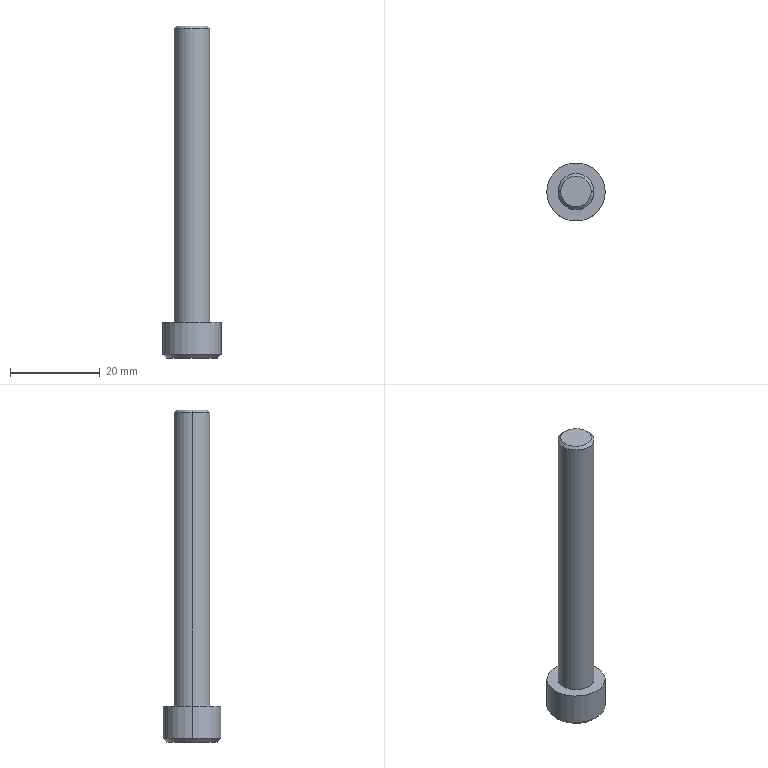Part | Creo | 1 solid | 18 faces | box 13 x 13 x 74 mm | volume 4213 mm3 | plane 10 | cylinder 4 | cone 4 | commonest cylinder face diameters 8 x2 13 x2
STEP:
#1=CARTESIAN_POINT('',(-106.5,-287.,8.5));
#2=VERTEX_POINT('',#1);
#3=CARTESIAN_POINT('',(-93.5,-287.,8.5));
#4=VERTEX_POINT('',#3);
#5=CARTESIAN_POINT('',(-100.,-287.,8.5));
#6=DIRECTION('',(0.,0.,1.));
#7=DIRECTION('',(-1.,0.,0.));
#8=AXIS2_PLACEMENT_3D('',#5,#6,#7);
#9=CIRCLE('',#8,6.5);
#10=EDGE_CURVE('',#2,#4,#9,.T.);
#11=ORIENTED_EDGE('',*,*,#10,.F.);
#12=CARTESIAN_POINT('',(-100.,-287.,8.5));
#13=DIRECTION('',(0.,0.,1.));
#14=DIRECTION('',(1.,0.,0.));
#15=AXIS2_PLACEMENT_3D('',#12,#13,#14);
#16=CIRCLE('',#15,6.5);
#17=EDGE_CURVE('',#4,#2,#16,.T.);
#18=ORIENTED_EDGE('',*,*,#17,.F.);
#19=EDGE_LOOP('',(#11,#18));
#20=FACE_OUTER_BOUND('',#19,.F.);
#21=CARTESIAN_POINT('',(-96.,-287.,8.5));
#22=VERTEX_POINT('',#21);
#23=CARTESIAN_POINT('',(-104.,-287.,8.5));
#24=VERTEX_POINT('',#23);
#25=CARTESIAN_POINT('',(-100.,-287.,8.5));
#26=DIRECTION('',(0.,0.,-1.));
#27=DIRECTION('',(1.,0.,0.));
#28=AXIS2_PLACEMENT_3D('',#25,#26,#27);
#29=CIRCLE('',#28,4.);
#30=EDGE_CURVE('',#22,#24,#29,.T.);
#31=ORIENTED_EDGE('',*,*,#30,.F.);
#32=CARTESIAN_POINT('',(-100.,-287.,8.5));
#33=DIRECTION('',(0.,0.,-1.));
#34=DIRECTION('',(-1.,0.,0.));
#35=AXIS2_PLACEMENT_3D('',#32,#33,#34);
#36=CIRCLE('',#35,4.);
#37=EDGE_CURVE('',#24,#22,#36,.T.);
#38=ORIENTED_EDGE('',*,*,#37,.F.);
#39=EDGE_LOOP('',(#31,#38));
#40=FACE_BOUND('',#39,.F.);
#41=CARTESIAN_POINT('',(-100.,-287.,8.5));
#42=DIRECTION('',(0.,0.,1.));
#43=DIRECTION('',(1.,0.,0.));
#44=AXIS2_PLACEMENT_3D('',#41,#42,#43);
#45=PLANE('',#44);
#46=ADVANCED_FACE('',(#20,#40),#45,.T.);
#47=CARTESIAN_POINT('',(-104.,-287.,73.9));
#48=VERTEX_POINT('',#47);
#49=CARTESIAN_POINT('',(-96.,-287.,73.9));
#50=VERTEX_POINT('',#49);
#51=CARTESIAN_POINT('',(-100.,-287.,73.9));
#52=DIRECTION('',(0.,0.,1.));
#53=DIRECTION('',(-1.,0.,0.));
#54=AXIS2_PLACEMENT_3D('',#51,#52,#53);
#55=CIRCLE('',#54,4.);
#56=EDGE_CURVE('',#48,#50,#55,.T.);
#57=ORIENTED_EDGE('',*,*,#56,.T.);
#58=CARTESIAN_POINT('',(-96.,-287.,8.5));
#59=DIRECTION('',(0.,0.,1.));
#60=VECTOR('',#59,65.4);
#61=LINE('',#58,#60);
#62=EDGE_CURVE('',#22,#50,#61,.T.);
#63=ORIENTED_EDGE('',*,*,#62,.F.);
#64=ORIENTED_EDGE('',*,*,#30,.T.);
#65=CARTESIAN_POINT('',(-104.,-287.,8.5));
#66=DIRECTION('',(0.,0.,1.));
#67=VECTOR('',#66,65.4);
#68=LINE('',#65,#67);
#69=EDGE_CURVE('',#24,#48,#68,.T.);
#70=ORIENTED_EDGE('',*,*,#69,.T.);
#71=EDGE_LOOP('',(#57,#63,#64,#70));
#72=FACE_OUTER_BOUND('',#71,.F.);
#73=CARTESIAN_POINT('',(-100.,-287.,-0.5));
#74=DIRECTION('',(0.,0.,1.));
#75=DIRECTION('',(1.,0.,0.));
#76=AXIS2_PLACEMENT_3D('',#73,#74,#75);
#77=CYLINDRICAL_SURFACE('',#76,4.);
#78=ADVANCED_FACE('',(#72),#77,.T.);
#79=CARTESIAN_POINT('',(-103.4,-287.,74.5));
#80=VERTEX_POINT('',#79);
#81=CARTESIAN_POINT('',(-96.6,-287.,74.5));
#82=VERTEX_POINT('',#81);
#83=CARTESIAN_POINT('',(-100.,-287.,74.5));
#84=DIRECTION('',(0.,0.,1.));
#85=DIRECTION('',(-1.,0.,0.));
#86=AXIS2_PLACEMENT_3D('',#83,#84,#85);
#87=CIRCLE('',#86,3.4);
#88=EDGE_CURVE('',#80,#82,#87,.T.);
#89=ORIENTED_EDGE('',*,*,#88,.T.);
#90=CARTESIAN_POINT('',(-96.6,-287.,74.5));
#91=DIRECTION('',(0.7071,0.,-0.7071));
#92=VECTOR('',#91,0.8485);
#93=LINE('',#90,#92);
#94=EDGE_CURVE('',#82,#50,#93,.T.);
#95=ORIENTED_EDGE('',*,*,#94,.T.);
#96=ORIENTED_EDGE('',*,*,#56,.F.);
#97=CARTESIAN_POINT('',(-103.4,-287.,74.5));
#98=DIRECTION('',(-0.7071,0.,-0.7071));
#99=VECTOR('',#98,0.8485);
#100=LINE('',#97,#99);
#101=EDGE_CURVE('',#80,#48,#100,.T.);
#102=ORIENTED_EDGE('',*,*,#101,.F.);
#103=EDGE_LOOP('',(#89,#95,#96,#102));
#104=FACE_OUTER_BOUND('',#103,.F.);
#105=CARTESIAN_POINT('',(-100.,-287.,74.2));
#106=DIRECTION('',(0.,0.,-1.));
#107=DIRECTION('',(-1.,0.,0.));
#108=AXIS2_PLACEMENT_3D('',#105,#106,#107);
#109=CONICAL_SURFACE('',#108,3.7,45.);
#110=ADVANCED_FACE('',(#104),#109,.T.);
#111=CARTESIAN_POINT('',(-100.,-287.,74.5));
#112=DIRECTION('',(0.,0.,1.));
#113=DIRECTION('',(1.,0.,0.));
#114=AXIS2_PLACEMENT_3D('',#111,#112,#113);
#115=CIRCLE('',#114,3.4);
#116=EDGE_CURVE('',#82,#80,#115,.T.);
#117=ORIENTED_EDGE('',*,*,#116,.F.);
#118=ORIENTED_EDGE('',*,*,#88,.F.);
#119=EDGE_LOOP('',(#117,#118));
#120=FACE_OUTER_BOUND('',#119,.F.);
#121=CARTESIAN_POINT('',(-100.,-287.,74.5));
#122=DIRECTION('',(0.,0.,1.));
#123=DIRECTION('',(1.,0.,0.));
#124=AXIS2_PLACEMENT_3D('',#121,#122,#123);
#125=PLANE('',#124);
#126=ADVANCED_FACE('',(#120),#125,.T.);
#127=ORIENTED_EDGE('',*,*,#116,.T.);
#128=ORIENTED_EDGE('',*,*,#101,.T.);
#129=CARTESIAN_POINT('',(-100.,-287.,73.9));
#130=DIRECTION('',(0.,0.,1.));
#131=DIRECTION('',(1.,0.,0.));
#132=AXIS2_PLACEMENT_3D('',#129,#130,#131);
#133=CIRCLE('',#132,4.);
#134=EDGE_CURVE('',#50,#48,#133,.T.);
#135=ORIENTED_EDGE('',*,*,#134,.F.);
#136=ORIENTED_EDGE('',*,*,#94,.F.);
#137=EDGE_LOOP('',(#127,#128,#135,#136));
#138=FACE_OUTER_BOUND('',#137,.F.);
#139=CARTESIAN_POINT('',(-100.,-287.,74.2));
#140=DIRECTION('',(0.,0.,-1.));
#141=DIRECTION('',(-1.,0.,0.));
#142=AXIS2_PLACEMENT_3D('',#139,#140,#141);
#143=CONICAL_SURFACE('',#142,3.7,45.);
#144=ADVANCED_FACE('',(#138),#143,.T.);
#145=ORIENTED_EDGE('',*,*,#134,.T.);
#146=ORIENTED_EDGE('',*,*,#69,.F.);
#147=ORIENTED_EDGE('',*,*,#37,.T.);
#148=ORIENTED_EDGE('',*,*,#62,.T.);
#149=EDGE_LOOP('',(#145,#146,#147,#148));
#150=FACE_OUTER_BOUND('',#149,.F.);
#151=CARTESIAN_POINT('',(-100.,-287.,-0.5));
#152=DIRECTION('',(0.,0.,1.));
#153=DIRECTION('',(1.,0.,0.));
#154=AXIS2_PLACEMENT_3D('',#151,#152,#153);
#155=CYLINDRICAL_SURFACE('',#154,4.);
#156=ADVANCED_FACE('',(#150),#155,.T.);
#157=CARTESIAN_POINT('',(-93.5,-287.,1.3));
#158=VERTEX_POINT('',#157);
#159=CARTESIAN_POINT('',(-106.5,-287.,1.3));
#160=VERTEX_POINT('',#159);
#161=CARTESIAN_POINT('',(-100.,-287.,1.3));
#162=DIRECTION('',(0.,0.,-1.));
#163=DIRECTION('',(1.,0.,0.));
#164=AXIS2_PLACEMENT_3D('',#161,#162,#163);
#165=CIRCLE('',#164,6.5);
#166=EDGE_CURVE('',#158,#160,#165,.T.);
#167=ORIENTED_EDGE('',*,*,#166,.T.);
#168=CARTESIAN_POINT('',(-106.5,-287.,1.3));
#169=DIRECTION('',(0.,0.,1.));
#170=VECTOR('',#169,7.2);
#171=LINE('',#168,#170);
#172=EDGE_CURVE('',#160,#2,#171,.T.);
#173=ORIENTED_EDGE('',*,*,#172,.T.);
#174=ORIENTED_EDGE('',*,*,#10,.T.);
#175=CARTESIAN_POINT('',(-93.5,-287.,1.3));
#176=DIRECTION('',(0.,0.,1.));
#177=VECTOR('',#176,7.2);
#178=LINE('',#175,#177);
#179=EDGE_CURVE('',#158,#4,#178,.T.);
#180=ORIENTED_EDGE('',*,*,#179,.F.);
#181=EDGE_LOOP('',(#167,#173,#174,#180));
#182=FACE_OUTER_BOUND('',#181,.F.);
#183=CARTESIAN_POINT('',(-100.,-287.,-0.5));
#184=DIRECTION('',(0.,0.,1.));
#185=DIRECTION('',(1.,0.,0.));
#186=AXIS2_PLACEMENT_3D('',#183,#184,#185);
#187=CYLINDRICAL_SURFACE('',#186,6.5);
#188=ADVANCED_FACE('',(#182),#187,.T.);
#189=CARTESIAN_POINT('',(-94.3,-287.,0.5));
#190=VERTEX_POINT('',#189);
#191=CARTESIAN_POINT('',(-105.7,-287.,0.5));
#192=VERTEX_POINT('',#191);
#193=CARTESIAN_POINT('',(-100.,-287.,0.5));
#194=DIRECTION('',(0.,0.,-1.));
#195=DIRECTION('',(1.,0.,0.));
#196=AXIS2_PLACEMENT_3D('',#193,#194,#195);
#197=CIRCLE('',#196,5.7);
#198=EDGE_CURVE('',#190,#192,#197,.T.);
#199=ORIENTED_EDGE('',*,*,#198,.T.);
#200=CARTESIAN_POINT('',(-105.7,-287.,0.5));
#201=DIRECTION('',(-0.7071,0.,0.7071));
#202=VECTOR('',#201,1.131);
#203=LINE('',#200,#202);
#204=EDGE_CURVE('',#192,#160,#203,.T.);
#205=ORIENTED_EDGE('',*,*,#204,.T.);
#206=ORIENTED_EDGE('',*,*,#166,.F.);
#207=CARTESIAN_POINT('',(-94.3,-287.,0.5));
#208=DIRECTION('',(0.7071,0.,0.7071));
#209=VECTOR('',#208,1.131);
#210=LINE('',#207,#209);
#211=EDGE_CURVE('',#190,#158,#210,.T.);
#212=ORIENTED_EDGE('',*,*,#211,.F.);
#213=EDGE_LOOP('',(#199,#205,#206,#212));
#214=FACE_OUTER_BOUND('',#213,.F.);
#215=CARTESIAN_POINT('',(-100.,-287.,0.9));
#216=DIRECTION('',(0.,0.,1.));
#217=DIRECTION('',(1.,0.,0.));
#218=AXIS2_PLACEMENT_3D('',#215,#216,#217);
#219=CONICAL_SURFACE('',#218,6.1,45.);
#220=ADVANCED_FACE('',(#214),#219,.T.);
#221=ORIENTED_EDGE('',*,*,#198,.F.);
#222=CARTESIAN_POINT('',(-100.,-287.,0.5));
#223=DIRECTION('',(0.,0.,-1.));
#224=DIRECTION('',(-1.,0.,0.));
#225=AXIS2_PLACEMENT_3D('',#222,#223,#224);
#226=CIRCLE('',#225,5.7);
#227=EDGE_CURVE('',#192,#190,#226,.T.);
#228=ORIENTED_EDGE('',*,*,#227,.F.);
#229=EDGE_LOOP('',(#221,#228));
#230=FACE_OUTER_BOUND('',#229,.F.);
#231=CARTESIAN_POINT('',(-103.,-288.732,0.5));
#232=VERTEX_POINT('',#231);
#233=CARTESIAN_POINT('',(-100.,-290.464,0.5));
#234=VERTEX_POINT('',#233);
#235=CARTESIAN_POINT('',(-103.,-288.732,0.5));
#236=DIRECTION('',(0.866,-0.5,0.));
#237=VECTOR('',#236,3.464);
#238=LINE('',#235,#237);
#239=EDGE_CURVE('',#232,#234,#238,.T.);
#240=ORIENTED_EDGE('',*,*,#239,.F.);
#241=CARTESIAN_POINT('',(-103.,-285.268,0.5));
#242=VERTEX_POINT('',#241);
#243=CARTESIAN_POINT('',(-103.,-285.268,0.5));
#244=DIRECTION('',(0.,-1.,0.));
#245=VECTOR('',#244,3.464);
#246=LINE('',#243,#245);
#247=EDGE_CURVE('',#242,#232,#246,.T.);
#248=ORIENTED_EDGE('',*,*,#247,.F.);
#249=CARTESIAN_POINT('',(-100.,-283.536,0.5));
#250=VERTEX_POINT('',#249);
#251=CARTESIAN_POINT('',(-100.,-283.536,0.5));
#252=DIRECTION('',(-0.866,-0.5,0.));
#253=VECTOR('',#252,3.464);
#254=LINE('',#251,#253);
#255=EDGE_CURVE('',#250,#242,#254,.T.);
#256=ORIENTED_EDGE('',*,*,#255,.F.);
#257=CARTESIAN_POINT('',(-97.,-285.268,0.5));
#258=VERTEX_POINT('',#257);
#259=CARTESIAN_POINT('',(-97.,-285.268,0.5));
#260=DIRECTION('',(-0.866,0.5,0.));
#261=VECTOR('',#260,3.464);
#262=LINE('',#259,#261);
#263=EDGE_CURVE('',#258,#250,#262,.T.);
#264=ORIENTED_EDGE('',*,*,#263,.F.);
#265=CARTESIAN_POINT('',(-97.,-288.732,0.5));
#266=VERTEX_POINT('',#265);
#267=CARTESIAN_POINT('',(-97.,-288.732,0.5));
#268=DIRECTION('',(0.,1.,0.));
#269=VECTOR('',#268,3.464);
#270=LINE('',#267,#269);
#271=EDGE_CURVE('',#266,#258,#270,.T.);
#272=ORIENTED_EDGE('',*,*,#271,.F.);
#273=CARTESIAN_POINT('',(-100.,-290.464,0.5));
#274=DIRECTION('',(0.866,0.5,0.));
#275=VECTOR('',#274,3.464);
#276=LINE('',#273,#275);
#277=EDGE_CURVE('',#234,#266,#276,.T.);
#278=ORIENTED_EDGE('',*,*,#277,.F.);
#279=EDGE_LOOP('',(#240,#248,#256,#264,#272,#278));
#280=FACE_BOUND('',#279,.F.);
#281=CARTESIAN_POINT('',(-100.,-287.,0.5));
#282=DIRECTION('',(0.,0.,1.));
#283=DIRECTION('',(1.,0.,0.));
#284=AXIS2_PLACEMENT_3D('',#281,#282,#283);
#285=PLANE('',#284);
#286=ADVANCED_FACE('',(#230,#280),#285,.F.);
#287=ORIENTED_EDGE('',*,*,#227,.T.);
#288=ORIENTED_EDGE('',*,*,#211,.T.);
#289=CARTESIAN_POINT('',(-100.,-287.,1.3));
#290=DIRECTION('',(0.,0.,-1.));
#291=DIRECTION('',(-1.,0.,0.));
#292=AXIS2_PLACEMENT_3D('',#289,#290,#291);
#293=CIRCLE('',#292,6.5);
#294=EDGE_CURVE('',#160,#158,#293,.T.);
#295=ORIENTED_EDGE('',*,*,#294,.F.);
#296=ORIENTED_EDGE('',*,*,#204,.F.);
#297=EDGE_LOOP('',(#287,#288,#295,#296));
#298=FACE_OUTER_BOUND('',#297,.F.);
#299=CARTESIAN_POINT('',(-100.,-287.,0.9));
#300=DIRECTION('',(0.,0.,1.));
#301=DIRECTION('',(1.,0.,0.));
#302=AXIS2_PLACEMENT_3D('',#299,#300,#301);
#303=CONICAL_SURFACE('',#302,6.1,45.);
#304=ADVANCED_FACE('',(#298),#303,.T.);
#305=ORIENTED_EDGE('',*,*,#294,.T.);
#306=ORIENTED_EDGE('',*,*,#179,.T.);
#307=ORIENTED_EDGE('',*,*,#17,.T.);
#308=ORIENTED_EDGE('',*,*,#172,.F.);
#309=EDGE_LOOP('',(#305,#306,#307,#308));
#310=FACE_OUTER_BOUND('',#309,.F.);
#311=CARTESIAN_POINT('',(-100.,-287.,-0.5));
#312=DIRECTION('',(0.,0.,1.));
#313=DIRECTION('',(1.,0.,0.));
#314=AXIS2_PLACEMENT_3D('',#311,#312,#313);
#315=CYLINDRICAL_SURFACE('',#314,6.5);
#316=ADVANCED_FACE('',(#310),#315,.T.);
#317=ORIENTED_EDGE('',*,*,#239,.T.);
#318=CARTESIAN_POINT('',(-100.,-290.464,5.3));
#319=VERTEX_POINT('',#318);
#320=CARTESIAN_POINT('',(-100.,-290.464,0.5));
#321=DIRECTION('',(0.,0.,1.));
#322=VECTOR('',#321,4.8);
#323=LINE('',#320,#322);
#324=EDGE_CURVE('',#234,#319,#323,.T.);
#325=ORIENTED_EDGE('',*,*,#324,.T.);
#326=CARTESIAN_POINT('',(-103.,-288.732,5.3));
#327=VERTEX_POINT('',#326);
#328=CARTESIAN_POINT('',(-100.,-290.464,5.3));
#329=DIRECTION('',(-0.866,0.5,0.));
#330=VECTOR('',#329,3.464);
#331=LINE('',#328,#330);
#332=EDGE_CURVE('',#319,#327,#331,.T.);
#333=ORIENTED_EDGE('',*,*,#332,.T.);
#334=CARTESIAN_POINT('',(-103.,-288.732,0.5));
#335=DIRECTION('',(0.,0.,1.));
#336=VECTOR('',#335,4.8);
#337=LINE('',#334,#336);
#338=EDGE_CURVE('',#232,#327,#337,.T.);
#339=ORIENTED_EDGE('',*,*,#338,.F.);
#340=EDGE_LOOP('',(#317,#325,#333,#339));
#341=FACE_OUTER_BOUND('',#340,.F.);
#342=CARTESIAN_POINT('',(-100.,-290.464,5.3));
#343=DIRECTION('',(-0.5,-0.866,0.));
#344=DIRECTION('',(0.866,-0.5,0.));
#345=AXIS2_PLACEMENT_3D('',#342,#343,#344);
#346=PLANE('',#345);
#347=ADVANCED_FACE('',(#341),#346,.F.);
#348=ORIENTED_EDGE('',*,*,#277,.T.);
#349=CARTESIAN_POINT('',(-97.,-288.732,5.3));
#350=VERTEX_POINT('',#349);
#351=CARTESIAN_POINT('',(-97.,-288.732,0.5));
#352=DIRECTION('',(0.,0.,1.));
#353=VECTOR('',#352,4.8);
#354=LINE('',#351,#353);
#355=EDGE_CURVE('',#266,#350,#354,.T.);
#356=ORIENTED_EDGE('',*,*,#355,.T.);
#357=CARTESIAN_POINT('',(-97.,-288.732,5.3));
#358=DIRECTION('',(-0.866,-0.5,0.));
#359=VECTOR('',#358,3.464);
#360=LINE('',#357,#359);
#361=EDGE_CURVE('',#350,#319,#360,.T.);
#362=ORIENTED_EDGE('',*,*,#361,.T.);
#363=ORIENTED_EDGE('',*,*,#324,.F.);
#364=EDGE_LOOP('',(#348,#356,#362,#363));
#365=FACE_OUTER_BOUND('',#364,.F.);
#366=CARTESIAN_POINT('',(-97.,-288.732,5.3));
#367=DIRECTION('',(0.5,-0.866,0.));
#368=DIRECTION('',(0.866,0.5,0.));
#369=AXIS2_PLACEMENT_3D('',#366,#367,#368);
#370=PLANE('',#369);
#371=ADVANCED_FACE('',(#365),#370,.F.);
#372=ORIENTED_EDGE('',*,*,#271,.T.);
#373=CARTESIAN_POINT('',(-97.,-285.268,5.3));
#374=VERTEX_POINT('',#373);
#375=CARTESIAN_POINT('',(-97.,-285.268,0.5));
#376=DIRECTION('',(0.,0.,1.));
#377=VECTOR('',#376,4.8);
#378=LINE('',#375,#377);
#379=EDGE_CURVE('',#258,#374,#378,.T.);
#380=ORIENTED_EDGE('',*,*,#379,.T.);
#381=CARTESIAN_POINT('',(-97.,-288.732,5.3));
#382=DIRECTION('',(0.,1.,0.));
#383=VECTOR('',#382,3.464);
#384=LINE('',#381,#383);
#385=EDGE_CURVE('',#350,#374,#384,.T.);
#386=ORIENTED_EDGE('',*,*,#385,.F.);
#387=ORIENTED_EDGE('',*,*,#355,.F.);
#388=EDGE_LOOP('',(#372,#380,#386,#387));
#389=FACE_OUTER_BOUND('',#388,.F.);
#390=CARTESIAN_POINT('',(-97.,-285.268,5.3));
#391=DIRECTION('',(1.,0.,0.));
#392=DIRECTION('',(0.,0.,-1.));
#393=AXIS2_PLACEMENT_3D('',#390,#391,#392);
#394=PLANE('',#393);
#395=ADVANCED_FACE('',(#389),#394,.F.);
#396=ORIENTED_EDGE('',*,*,#263,.T.);
#397=CARTESIAN_POINT('',(-100.,-283.536,5.3));
#398=VERTEX_POINT('',#397);
#399=CARTESIAN_POINT('',(-100.,-283.536,0.5));
#400=DIRECTION('',(0.,0.,1.));
#401=VECTOR('',#400,4.8);
#402=LINE('',#399,#401);
#403=EDGE_CURVE('',#250,#398,#402,.T.);
#404=ORIENTED_EDGE('',*,*,#403,.T.);
#405=CARTESIAN_POINT('',(-100.,-283.536,5.3));
#406=DIRECTION('',(0.866,-0.5,0.));
#407=VECTOR('',#406,3.464);
#408=LINE('',#405,#407);
#409=EDGE_CURVE('',#398,#374,#408,.T.);
#410=ORIENTED_EDGE('',*,*,#409,.T.);
#411=ORIENTED_EDGE('',*,*,#379,.F.);
#412=EDGE_LOOP('',(#396,#404,#410,#411));
#413=FACE_OUTER_BOUND('',#412,.F.);
#414=CARTESIAN_POINT('',(-100.,-283.536,5.3));
#415=DIRECTION('',(0.5,0.866,0.));
#416=DIRECTION('',(-0.866,0.5,0.));
#417=AXIS2_PLACEMENT_3D('',#414,#415,#416);
#418=PLANE('',#417);
#419=ADVANCED_FACE('',(#413),#418,.F.);
#420=ORIENTED_EDGE('',*,*,#255,.T.);
#421=CARTESIAN_POINT('',(-103.,-285.268,5.3));
#422=VERTEX_POINT('',#421);
#423=CARTESIAN_POINT('',(-103.,-285.268,0.5));
#424=DIRECTION('',(0.,0.,1.));
#425=VECTOR('',#424,4.8);
#426=LINE('',#423,#425);
#427=EDGE_CURVE('',#242,#422,#426,.T.);
#428=ORIENTED_EDGE('',*,*,#427,.T.);
#429=CARTESIAN_POINT('',(-103.,-285.268,5.3));
#430=DIRECTION('',(0.866,0.5,0.));
#431=VECTOR('',#430,3.464);
#432=LINE('',#429,#431);
#433=EDGE_CURVE('',#422,#398,#432,.T.);
#434=ORIENTED_EDGE('',*,*,#433,.T.);
#435=ORIENTED_EDGE('',*,*,#403,.F.);
#436=EDGE_LOOP('',(#420,#428,#434,#435));
#437=FACE_OUTER_BOUND('',#436,.F.);
#438=CARTESIAN_POINT('',(-103.,-285.268,5.3));
#439=DIRECTION('',(-0.5,0.866,0.));
#440=DIRECTION('',(-0.866,-0.5,0.));
#441=AXIS2_PLACEMENT_3D('',#438,#439,#440);
#442=PLANE('',#441);
#443=ADVANCED_FACE('',(#437),#442,.F.);
#444=ORIENTED_EDGE('',*,*,#247,.T.);
#445=ORIENTED_EDGE('',*,*,#338,.T.);
#446=CARTESIAN_POINT('',(-103.,-285.268,5.3));
#447=DIRECTION('',(0.,-1.,0.));
#448=VECTOR('',#447,3.464);
#449=LINE('',#446,#448);
#450=EDGE_CURVE('',#422,#327,#449,.T.);
#451=ORIENTED_EDGE('',*,*,#450,.F.);
#452=ORIENTED_EDGE('',*,*,#427,.F.);
#453=EDGE_LOOP('',(#444,#445,#451,#452));
#454=FACE_OUTER_BOUND('',#453,.F.);
#455=CARTESIAN_POINT('',(-103.,-288.732,5.3));
#456=DIRECTION('',(-1.,0.,0.));
#457=DIRECTION('',(0.,0.,1.));
#458=AXIS2_PLACEMENT_3D('',#455,#456,#457);
#459=PLANE('',#458);
#460=ADVANCED_FACE('',(#454),#459,.F.);
#461=ORIENTED_EDGE('',*,*,#361,.F.);
#462=ORIENTED_EDGE('',*,*,#385,.T.);
#463=ORIENTED_EDGE('',*,*,#409,.F.);
#464=ORIENTED_EDGE('',*,*,#433,.F.);
#465=ORIENTED_EDGE('',*,*,#450,.T.);
#466=ORIENTED_EDGE('',*,*,#332,.F.);
#467=EDGE_LOOP('',(#461,#462,#463,#464,#465,#466));
#468=FACE_OUTER_BOUND('',#467,.F.);
#469=CARTESIAN_POINT('',(-103.,-292.196,5.3));
#470=DIRECTION('',(0.,0.,-1.));
#471=DIRECTION('',(-1.,0.,0.));
#472=AXIS2_PLACEMENT_3D('',#469,#470,#471);
#473=PLANE('',#472);
#474=ADVANCED_FACE('',(#468),#473,.T.);
#475=CLOSED_SHELL('',(#46,#78,#110,#126,#144,#156,#188,#220,#286,#304,#316,#347,#371,#395,#419,#443,#460,#474));
#476=MANIFOLD_SOLID_BREP('',#475);
#477=(LENGTH_UNIT()NAMED_UNIT(*)SI_UNIT(.MILLI.,.METRE.));
#478=UNCERTAINTY_MEASURE_WITH_UNIT(LENGTH_MEASURE(0.007625),#477,'','');
#479=(NAMED_UNIT(*)PLANE_ANGLE_UNIT()SI_UNIT($,.RADIAN.));
#480=PLANE_ANGLE_MEASURE_WITH_UNIT(PLANE_ANGLE_MEASURE(0.01745),#479);
#481=(CONVERSION_BASED_UNIT('DEGREE',#480)NAMED_UNIT(*)PLANE_ANGLE_UNIT());
#482=(NAMED_UNIT(*)SI_UNIT($,.STERADIAN.)SOLID_ANGLE_UNIT());
#483=(GEOMETRIC_REPRESENTATION_CONTEXT(3)GLOBAL_UNCERTAINTY_ASSIGNED_CONTEXT((#478))GLOBAL_UNIT_ASSIGNED_CONTEXT((#477,#481,#482))REPRESENTATION_CONTEXT('',''));
#484=ADVANCED_BREP_SHAPE_REPRESENTATION('',(#476),#483);